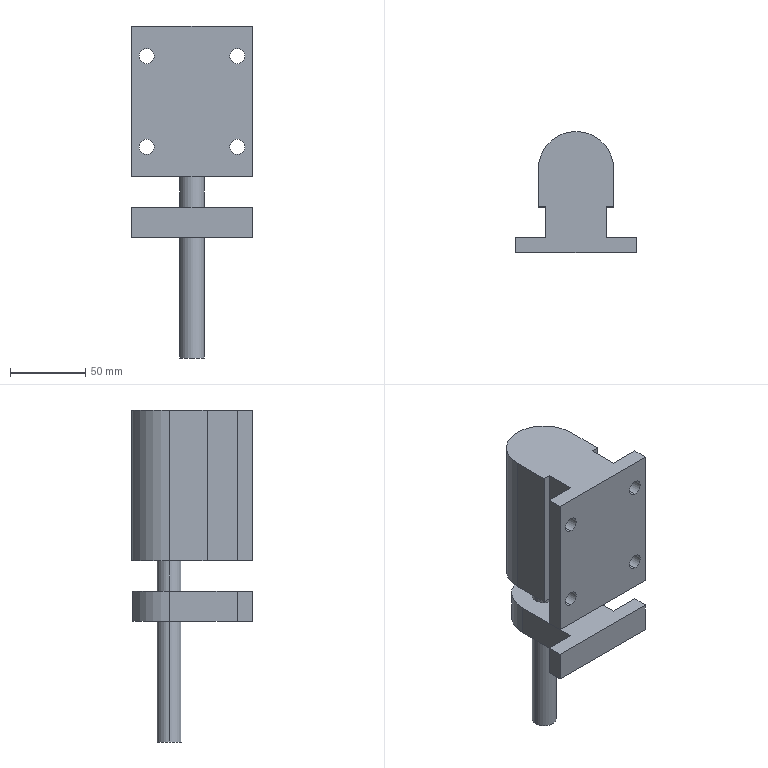Part | SolidWorks | features BaseBody 1 | 1 solid | 39 faces | box 80 x 80 x 220 mm | volume 466808 mm3 | plane 23 | cylinder 16 | commonest cylinder face diameters 10 x8 16 x4 50 x4
STEP:
#1=CARTESIAN_POINT('',(-246.782,7.138,175.));
#2=VERTEX_POINT('',#1);
#3=CARTESIAN_POINT('',(-246.782,7.138,165.));
#4=VERTEX_POINT('',#3);
#5=CARTESIAN_POINT('',(-246.782,7.138,170.));
#6=DIRECTION('',(0.,-1.,0.));
#7=DIRECTION('',(0.,0.,1.));
#8=AXIS2_PLACEMENT_3D('',#5,#6,#7);
#9=CIRCLE('',#8,5.);
#10=EDGE_CURVE('',#2,#4,#9,.T.);
#11=ORIENTED_EDGE('',*,*,#10,.T.);
#12=CARTESIAN_POINT('',(-246.782,17.138,165.));
#13=VERTEX_POINT('',#12);
#14=CARTESIAN_POINT('',(-246.782,-2.862,165.));
#15=DIRECTION('',(0.,1.,0.));
#16=VECTOR('',#15,1000.);
#17=LINE('',#14,#16);
#18=EDGE_CURVE('',#4,#13,#17,.T.);
#19=ORIENTED_EDGE('',*,*,#18,.T.);
#20=CARTESIAN_POINT('',(-246.782,17.138,175.));
#21=VERTEX_POINT('',#20);
#22=CARTESIAN_POINT('',(-246.782,17.138,170.));
#23=DIRECTION('',(0.,1.,0.));
#24=DIRECTION('',(0.,0.,1.));
#25=AXIS2_PLACEMENT_3D('',#22,#23,#24);
#26=CIRCLE('',#25,5.);
#27=EDGE_CURVE('',#13,#21,#26,.T.);
#28=ORIENTED_EDGE('',*,*,#27,.T.);
#29=CARTESIAN_POINT('',(-246.782,-2.862,175.));
#30=DIRECTION('',(0.,1.,0.));
#31=VECTOR('',#30,1000.);
#32=LINE('',#29,#31);
#33=EDGE_CURVE('',#2,#21,#32,.T.);
#34=ORIENTED_EDGE('',*,*,#33,.F.);
#35=EDGE_LOOP('',(#11,#19,#28,#34));
#36=FACE_OUTER_BOUND('',#35,.T.);
#37=CARTESIAN_POINT('',(-246.782,-2.862,170.));
#38=DIRECTION('',(0.,1.,0.));
#39=DIRECTION('',(0.,0.,1.));
#40=AXIS2_PLACEMENT_3D('',#37,#38,#39);
#41=CYLINDRICAL_SURFACE('',#40,5.);
#42=ADVANCED_FACE('',(#36),#41,.F.);
#43=CARTESIAN_POINT('',(-246.782,7.138,115.));
#44=VERTEX_POINT('',#43);
#45=CARTESIAN_POINT('',(-246.782,7.138,105.));
#46=VERTEX_POINT('',#45);
#47=CARTESIAN_POINT('',(-246.782,7.138,110.));
#48=DIRECTION('',(0.,-1.,0.));
#49=DIRECTION('',(0.,0.,1.));
#50=AXIS2_PLACEMENT_3D('',#47,#48,#49);
#51=CIRCLE('',#50,5.);
#52=EDGE_CURVE('',#44,#46,#51,.T.);
#53=ORIENTED_EDGE('',*,*,#52,.T.);
#54=CARTESIAN_POINT('',(-246.782,17.138,105.));
#55=VERTEX_POINT('',#54);
#56=CARTESIAN_POINT('',(-246.782,-2.862,105.));
#57=DIRECTION('',(0.,1.,0.));
#58=VECTOR('',#57,1000.);
#59=LINE('',#56,#58);
#60=EDGE_CURVE('',#46,#55,#59,.T.);
#61=ORIENTED_EDGE('',*,*,#60,.T.);
#62=CARTESIAN_POINT('',(-246.782,17.138,115.));
#63=VERTEX_POINT('',#62);
#64=CARTESIAN_POINT('',(-246.782,17.138,110.));
#65=DIRECTION('',(0.,1.,0.));
#66=DIRECTION('',(0.,0.,1.));
#67=AXIS2_PLACEMENT_3D('',#64,#65,#66);
#68=CIRCLE('',#67,5.);
#69=EDGE_CURVE('',#55,#63,#68,.T.);
#70=ORIENTED_EDGE('',*,*,#69,.T.);
#71=CARTESIAN_POINT('',(-246.782,-2.862,115.));
#72=DIRECTION('',(0.,1.,0.));
#73=VECTOR('',#72,1000.);
#74=LINE('',#71,#73);
#75=EDGE_CURVE('',#44,#63,#74,.T.);
#76=ORIENTED_EDGE('',*,*,#75,.F.);
#77=EDGE_LOOP('',(#53,#61,#70,#76));
#78=FACE_OUTER_BOUND('',#77,.T.);
#79=CARTESIAN_POINT('',(-246.782,-2.862,110.));
#80=DIRECTION('',(0.,1.,0.));
#81=DIRECTION('',(0.,0.,1.));
#82=AXIS2_PLACEMENT_3D('',#79,#80,#81);
#83=CYLINDRICAL_SURFACE('',#82,5.);
#84=ADVANCED_FACE('',(#78),#83,.F.);
#85=CARTESIAN_POINT('',(-306.782,7.138,115.));
#86=VERTEX_POINT('',#85);
#87=CARTESIAN_POINT('',(-306.782,7.138,105.));
#88=VERTEX_POINT('',#87);
#89=CARTESIAN_POINT('',(-306.782,7.138,110.));
#90=DIRECTION('',(0.,-1.,0.));
#91=DIRECTION('',(0.,0.,1.));
#92=AXIS2_PLACEMENT_3D('',#89,#90,#91);
#93=CIRCLE('',#92,5.);
#94=EDGE_CURVE('',#86,#88,#93,.T.);
#95=ORIENTED_EDGE('',*,*,#94,.T.);
#96=CARTESIAN_POINT('',(-306.782,17.138,105.));
#97=VERTEX_POINT('',#96);
#98=CARTESIAN_POINT('',(-306.782,-2.862,105.));
#99=DIRECTION('',(0.,1.,0.));
#100=VECTOR('',#99,1000.);
#101=LINE('',#98,#100);
#102=EDGE_CURVE('',#88,#97,#101,.T.);
#103=ORIENTED_EDGE('',*,*,#102,.T.);
#104=CARTESIAN_POINT('',(-306.782,17.138,115.));
#105=VERTEX_POINT('',#104);
#106=CARTESIAN_POINT('',(-306.782,17.138,110.));
#107=DIRECTION('',(0.,1.,0.));
#108=DIRECTION('',(0.,0.,-1.));
#109=AXIS2_PLACEMENT_3D('',#106,#107,#108);
#110=CIRCLE('',#109,5.);
#111=EDGE_CURVE('',#97,#105,#110,.T.);
#112=ORIENTED_EDGE('',*,*,#111,.T.);
#113=CARTESIAN_POINT('',(-306.782,-2.862,115.));
#114=DIRECTION('',(0.,1.,0.));
#115=VECTOR('',#114,1000.);
#116=LINE('',#113,#115);
#117=EDGE_CURVE('',#86,#105,#116,.T.);
#118=ORIENTED_EDGE('',*,*,#117,.F.);
#119=EDGE_LOOP('',(#95,#103,#112,#118));
#120=FACE_OUTER_BOUND('',#119,.T.);
#121=CARTESIAN_POINT('',(-306.782,-2.862,110.));
#122=DIRECTION('',(0.,1.,0.));
#123=DIRECTION('',(0.,0.,1.));
#124=AXIS2_PLACEMENT_3D('',#121,#122,#123);
#125=CYLINDRICAL_SURFACE('',#124,5.);
#126=ADVANCED_FACE('',(#120),#125,.F.);
#127=CARTESIAN_POINT('',(-306.782,7.138,175.));
#128=VERTEX_POINT('',#127);
#129=CARTESIAN_POINT('',(-306.782,7.138,165.));
#130=VERTEX_POINT('',#129);
#131=CARTESIAN_POINT('',(-306.782,7.138,170.));
#132=DIRECTION('',(0.,-1.,0.));
#133=DIRECTION('',(0.,0.,1.));
#134=AXIS2_PLACEMENT_3D('',#131,#132,#133);
#135=CIRCLE('',#134,5.);
#136=EDGE_CURVE('',#128,#130,#135,.T.);
#137=ORIENTED_EDGE('',*,*,#136,.T.);
#138=CARTESIAN_POINT('',(-306.782,17.138,165.));
#139=VERTEX_POINT('',#138);
#140=CARTESIAN_POINT('',(-306.782,-2.862,165.));
#141=DIRECTION('',(0.,1.,0.));
#142=VECTOR('',#141,1000.);
#143=LINE('',#140,#142);
#144=EDGE_CURVE('',#130,#139,#143,.T.);
#145=ORIENTED_EDGE('',*,*,#144,.T.);
#146=CARTESIAN_POINT('',(-306.782,17.138,175.));
#147=VERTEX_POINT('',#146);
#148=CARTESIAN_POINT('',(-306.782,17.138,170.));
#149=DIRECTION('',(0.,1.,0.));
#150=DIRECTION('',(0.,0.,-1.));
#151=AXIS2_PLACEMENT_3D('',#148,#149,#150);
#152=CIRCLE('',#151,5.);
#153=EDGE_CURVE('',#139,#147,#152,.T.);
#154=ORIENTED_EDGE('',*,*,#153,.T.);
#155=CARTESIAN_POINT('',(-306.782,-2.862,175.));
#156=DIRECTION('',(0.,1.,0.));
#157=VECTOR('',#156,1000.);
#158=LINE('',#155,#157);
#159=EDGE_CURVE('',#128,#147,#158,.T.);
#160=ORIENTED_EDGE('',*,*,#159,.F.);
#161=EDGE_LOOP('',(#137,#145,#154,#160));
#162=FACE_OUTER_BOUND('',#161,.T.);
#163=CARTESIAN_POINT('',(-306.782,-2.862,170.));
#164=DIRECTION('',(0.,1.,0.));
#165=DIRECTION('',(0.,0.,1.));
#166=AXIS2_PLACEMENT_3D('',#163,#164,#165);
#167=CYLINDRICAL_SURFACE('',#166,5.);
#168=ADVANCED_FACE('',(#162),#167,.F.);
#169=CARTESIAN_POINT('',(-284.782,62.138,90.));
#170=VERTEX_POINT('',#169);
#171=CARTESIAN_POINT('',(-268.782,62.138,90.));
#172=VERTEX_POINT('',#171);
#173=CARTESIAN_POINT('',(-276.782,62.138,90.));
#174=DIRECTION('',(0.,0.,-1.));
#175=DIRECTION('',(1.,0.,0.));
#176=AXIS2_PLACEMENT_3D('',#173,#174,#175);
#177=CIRCLE('',#176,8.);
#178=EDGE_CURVE('',#170,#172,#177,.T.);
#179=ORIENTED_EDGE('',*,*,#178,.T.);
#180=CARTESIAN_POINT('',(-268.782,62.138,70.));
#181=VERTEX_POINT('',#180);
#182=CARTESIAN_POINT('',(-268.782,62.138,112.627));
#183=DIRECTION('',(0.,0.,-1.));
#184=VECTOR('',#183,1000.);
#185=LINE('',#182,#184);
#186=EDGE_CURVE('',#172,#181,#185,.T.);
#187=ORIENTED_EDGE('',*,*,#186,.T.);
#188=CARTESIAN_POINT('',(-284.782,62.138,70.));
#189=VERTEX_POINT('',#188);
#190=CARTESIAN_POINT('',(-276.782,62.138,70.));
#191=DIRECTION('',(0.,0.,-1.));
#192=DIRECTION('',(-1.,0.,0.));
#193=AXIS2_PLACEMENT_3D('',#190,#191,#192);
#194=CIRCLE('',#193,8.);
#195=EDGE_CURVE('',#189,#181,#194,.T.);
#196=ORIENTED_EDGE('',*,*,#195,.F.);
#197=CARTESIAN_POINT('',(-284.782,62.138,112.627));
#198=DIRECTION('',(0.,0.,-1.));
#199=VECTOR('',#198,1000.);
#200=LINE('',#197,#199);
#201=EDGE_CURVE('',#170,#189,#200,.T.);
#202=ORIENTED_EDGE('',*,*,#201,.F.);
#203=EDGE_LOOP('',(#179,#187,#196,#202));
#204=FACE_OUTER_BOUND('',#203,.T.);
#205=CARTESIAN_POINT('',(-276.782,62.138,112.627));
#206=DIRECTION('',(0.,0.,-1.));
#207=DIRECTION('',(-1.,0.,0.));
#208=AXIS2_PLACEMENT_3D('',#205,#206,#207);
#209=CYLINDRICAL_SURFACE('',#208,8.);
#210=ADVANCED_FACE('',(#204),#209,.T.);
#211=CARTESIAN_POINT('',(-284.782,62.138,-30.));
#212=VERTEX_POINT('',#211);
#213=CARTESIAN_POINT('',(-268.782,62.138,-30.));
#214=VERTEX_POINT('',#213);
#215=CARTESIAN_POINT('',(-276.782,62.138,-30.));
#216=DIRECTION('',(0.,0.,-1.));
#217=DIRECTION('',(-1.,0.,0.));
#218=AXIS2_PLACEMENT_3D('',#215,#216,#217);
#219=CIRCLE('',#218,8.);
#220=EDGE_CURVE('',#212,#214,#219,.T.);
#221=ORIENTED_EDGE('',*,*,#220,.F.);
#222=CARTESIAN_POINT('',(-284.782,62.138,50.));
#223=VERTEX_POINT('',#222);
#224=CARTESIAN_POINT('',(-284.782,62.138,-30.));
#225=DIRECTION('',(0.,0.,1.));
#226=VECTOR('',#225,1000.);
#227=LINE('',#224,#226);
#228=EDGE_CURVE('',#212,#223,#227,.T.);
#229=ORIENTED_EDGE('',*,*,#228,.T.);
#230=CARTESIAN_POINT('',(-268.782,62.138,50.));
#231=VERTEX_POINT('',#230);
#232=CARTESIAN_POINT('',(-276.782,62.138,50.));
#233=DIRECTION('',(0.,0.,-1.));
#234=DIRECTION('',(1.,0.,0.));
#235=AXIS2_PLACEMENT_3D('',#232,#233,#234);
#236=CIRCLE('',#235,8.);
#237=EDGE_CURVE('',#223,#231,#236,.T.);
#238=ORIENTED_EDGE('',*,*,#237,.T.);
#239=CARTESIAN_POINT('',(-268.782,62.138,-30.));
#240=DIRECTION('',(0.,0.,1.));
#241=VECTOR('',#240,1000.);
#242=LINE('',#239,#241);
#243=EDGE_CURVE('',#214,#231,#242,.T.);
#244=ORIENTED_EDGE('',*,*,#243,.F.);
#245=EDGE_LOOP('',(#221,#229,#238,#244));
#246=FACE_OUTER_BOUND('',#245,.T.);
#247=CARTESIAN_POINT('',(-276.782,62.138,-30.));
#248=DIRECTION('',(0.,0.,1.));
#249=DIRECTION('',(1.,0.,0.));
#250=AXIS2_PLACEMENT_3D('',#247,#248,#249);
#251=CYLINDRICAL_SURFACE('',#250,8.);
#252=ADVANCED_FACE('',(#246),#251,.T.);
#253=CARTESIAN_POINT('',(-276.782,62.138,-30.));
#254=DIRECTION('',(0.,0.,-1.));
#255=DIRECTION('',(-1.,0.,0.));
#256=AXIS2_PLACEMENT_3D('',#253,#254,#255);
#257=CIRCLE('',#256,8.);
#258=EDGE_CURVE('',#214,#212,#257,.T.);
#259=ORIENTED_EDGE('',*,*,#258,.T.);
#260=ORIENTED_EDGE('',*,*,#220,.T.);
#261=EDGE_LOOP('',(#259,#260));
#262=FACE_OUTER_BOUND('',#261,.T.);
#263=CARTESIAN_POINT('',(-276.782,62.138,-30.));
#264=DIRECTION('',(0.,0.,-1.));
#265=DIRECTION('',(-1.,0.,0.));
#266=AXIS2_PLACEMENT_3D('',#263,#264,#265);
#267=PLANE('',#266);
#268=ADVANCED_FACE('',(#262),#267,.T.);
#269=ORIENTED_EDGE('',*,*,#228,.F.);
#270=ORIENTED_EDGE('',*,*,#258,.F.);
#271=ORIENTED_EDGE('',*,*,#243,.T.);
#272=CARTESIAN_POINT('',(-276.782,62.138,50.));
#273=DIRECTION('',(0.,0.,-1.));
#274=DIRECTION('',(1.,0.,0.));
#275=AXIS2_PLACEMENT_3D('',#272,#273,#274);
#276=CIRCLE('',#275,8.);
#277=EDGE_CURVE('',#231,#223,#276,.T.);
#278=ORIENTED_EDGE('',*,*,#277,.T.);
#279=EDGE_LOOP('',(#269,#270,#271,#278));
#280=FACE_OUTER_BOUND('',#279,.T.);
#281=CARTESIAN_POINT('',(-276.782,62.138,-30.));
#282=DIRECTION('',(0.,0.,1.));
#283=DIRECTION('',(1.,0.,0.));
#284=AXIS2_PLACEMENT_3D('',#281,#282,#283);
#285=CYLINDRICAL_SURFACE('',#284,8.);
#286=ADVANCED_FACE('',(#280),#285,.T.);
#287=CARTESIAN_POINT('',(-296.782,37.138,90.));
#288=VERTEX_POINT('',#287);
#289=CARTESIAN_POINT('',(-301.782,37.138,90.));
#290=VERTEX_POINT('',#289);
#291=CARTESIAN_POINT('',(-251.782,37.138,90.));
#292=DIRECTION('',(-1.,0.,0.));
#293=VECTOR('',#292,1000.);
#294=LINE('',#291,#293);
#295=EDGE_CURVE('',#288,#290,#294,.T.);
#296=ORIENTED_EDGE('',*,*,#295,.F.);
#297=CARTESIAN_POINT('',(-296.782,37.138,190.));
#298=VERTEX_POINT('',#297);
#299=CARTESIAN_POINT('',(-296.782,37.138,190.));
#300=DIRECTION('',(0.,0.,1.));
#301=VECTOR('',#300,1000.);
#302=LINE('',#299,#301);
#303=EDGE_CURVE('',#288,#298,#302,.T.);
#304=ORIENTED_EDGE('',*,*,#303,.T.);
#305=CARTESIAN_POINT('',(-301.782,37.138,190.));
#306=VERTEX_POINT('',#305);
#307=CARTESIAN_POINT('',(-301.782,37.138,190.));
#308=DIRECTION('',(1.,0.,0.));
#309=VECTOR('',#308,1000.);
#310=LINE('',#307,#309);
#311=EDGE_CURVE('',#306,#298,#310,.T.);
#312=ORIENTED_EDGE('',*,*,#311,.F.);
#313=CARTESIAN_POINT('',(-301.782,37.138,90.));
#314=DIRECTION('',(0.,0.,1.));
#315=VECTOR('',#314,1000.);
#316=LINE('',#313,#315);
#317=EDGE_CURVE('',#290,#306,#316,.T.);
#318=ORIENTED_EDGE('',*,*,#317,.F.);
#319=EDGE_LOOP('',(#296,#304,#312,#318));
#320=FACE_OUTER_BOUND('',#319,.T.);
#321=CARTESIAN_POINT('',(-616.782,37.138,0.));
#322=DIRECTION('',(0.,1.,0.));
#323=DIRECTION('',(0.,0.,1.));
#324=AXIS2_PLACEMENT_3D('',#321,#322,#323);
#325=PLANE('',#324);
#326=ADVANCED_FACE('',(#320),#325,.F.);
#327=CARTESIAN_POINT('',(-296.782,17.138,90.));
#328=VERTEX_POINT('',#327);
#329=CARTESIAN_POINT('',(-296.782,17.138,190.));
#330=VERTEX_POINT('',#329);
#331=CARTESIAN_POINT('',(-296.782,17.138,190.));
#332=DIRECTION('',(0.,0.,1.));
#333=VECTOR('',#332,1000.);
#334=LINE('',#331,#333);
#335=EDGE_CURVE('',#328,#330,#334,.T.);
#336=ORIENTED_EDGE('',*,*,#335,.T.);
#337=CARTESIAN_POINT('',(-296.782,37.138,190.));
#338=DIRECTION('',(0.,-1.,0.));
#339=VECTOR('',#338,1000.);
#340=LINE('',#337,#339);
#341=EDGE_CURVE('',#298,#330,#340,.T.);
#342=ORIENTED_EDGE('',*,*,#341,.F.);
#343=ORIENTED_EDGE('',*,*,#303,.F.);
#344=CARTESIAN_POINT('',(-296.782,37.138,90.));
#345=DIRECTION('',(0.,-1.,0.));
#346=VECTOR('',#345,1000.);
#347=LINE('',#344,#346);
#348=EDGE_CURVE('',#288,#328,#347,.T.);
#349=ORIENTED_EDGE('',*,*,#348,.T.);
#350=EDGE_LOOP('',(#336,#342,#343,#349));
#351=FACE_OUTER_BOUND('',#350,.T.);
#352=CARTESIAN_POINT('',(-296.782,37.138,190.));
#353=DIRECTION('',(1.,0.,0.));
#354=DIRECTION('',(0.,0.,-1.));
#355=AXIS2_PLACEMENT_3D('',#352,#353,#354);
#356=PLANE('',#355);
#357=ADVANCED_FACE('',(#351),#356,.F.);
#358=CARTESIAN_POINT('',(-256.782,17.138,190.));
#359=VERTEX_POINT('',#358);
#360=CARTESIAN_POINT('',(-256.782,17.138,90.));
#361=VERTEX_POINT('',#360);
#362=CARTESIAN_POINT('',(-256.782,17.138,90.));
#363=DIRECTION('',(0.,0.,-1.));
#364=VECTOR('',#363,1000.);
#365=LINE('',#362,#364);
#366=EDGE_CURVE('',#359,#361,#365,.T.);
#367=ORIENTED_EDGE('',*,*,#366,.T.);
#368=CARTESIAN_POINT('',(-256.782,37.138,90.));
#369=VERTEX_POINT('',#368);
#370=CARTESIAN_POINT('',(-256.782,37.138,90.));
#371=DIRECTION('',(0.,-1.,0.));
#372=VECTOR('',#371,1000.);
#373=LINE('',#370,#372);
#374=EDGE_CURVE('',#369,#361,#373,.T.);
#375=ORIENTED_EDGE('',*,*,#374,.F.);
#376=CARTESIAN_POINT('',(-256.782,37.138,190.));
#377=VERTEX_POINT('',#376);
#378=CARTESIAN_POINT('',(-256.782,37.138,90.));
#379=DIRECTION('',(0.,0.,-1.));
#380=VECTOR('',#379,1000.);
#381=LINE('',#378,#380);
#382=EDGE_CURVE('',#377,#369,#381,.T.);
#383=ORIENTED_EDGE('',*,*,#382,.F.);
#384=CARTESIAN_POINT('',(-256.782,37.138,190.));
#385=DIRECTION('',(0.,-1.,0.));
#386=VECTOR('',#385,1000.);
#387=LINE('',#384,#386);
#388=EDGE_CURVE('',#377,#359,#387,.T.);
#389=ORIENTED_EDGE('',*,*,#388,.T.);
#390=EDGE_LOOP('',(#367,#375,#383,#389));
#391=FACE_OUTER_BOUND('',#390,.T.);
#392=CARTESIAN_POINT('',(-256.782,37.138,90.));
#393=DIRECTION('',(-1.,0.,0.));
#394=DIRECTION('',(0.,0.,1.));
#395=AXIS2_PLACEMENT_3D('',#392,#393,#394);
#396=PLANE('',#395);
#397=ADVANCED_FACE('',(#391),#396,.F.);
#398=CARTESIAN_POINT('',(-251.782,37.138,190.));
#399=VERTEX_POINT('',#398);
#400=CARTESIAN_POINT('',(-301.782,37.138,190.));
#401=DIRECTION('',(1.,0.,0.));
#402=VECTOR('',#401,1000.);
#403=LINE('',#400,#402);
#404=EDGE_CURVE('',#377,#399,#403,.T.);
#405=ORIENTED_EDGE('',*,*,#404,.F.);
#406=ORIENTED_EDGE('',*,*,#382,.T.);
#407=CARTESIAN_POINT('',(-251.782,37.138,90.));
#408=VERTEX_POINT('',#407);
#409=CARTESIAN_POINT('',(-251.782,37.138,90.));
#410=DIRECTION('',(-1.,0.,0.));
#411=VECTOR('',#410,1000.);
#412=LINE('',#409,#411);
#413=EDGE_CURVE('',#408,#369,#412,.T.);
#414=ORIENTED_EDGE('',*,*,#413,.F.);
#415=CARTESIAN_POINT('',(-251.782,37.138,190.));
#416=DIRECTION('',(0.,0.,-1.));
#417=VECTOR('',#416,1000.);
#418=LINE('',#415,#417);
#419=EDGE_CURVE('',#399,#408,#418,.T.);
#420=ORIENTED_EDGE('',*,*,#419,.F.);
#421=EDGE_LOOP('',(#405,#406,#414,#420));
#422=FACE_OUTER_BOUND('',#421,.T.);
#423=CARTESIAN_POINT('',(-616.782,37.138,0.));
#424=DIRECTION('',(0.,1.,0.));
#425=DIRECTION('',(0.,0.,1.));
#426=AXIS2_PLACEMENT_3D('',#423,#424,#425);
#427=PLANE('',#426);
#428=ADVANCED_FACE('',(#422),#427,.F.);
#429=CARTESIAN_POINT('',(-251.782,62.138,90.));
#430=VERTEX_POINT('',#429);
#431=CARTESIAN_POINT('',(-251.782,87.138,90.));
#432=DIRECTION('',(0.,-1.,0.));
#433=VECTOR('',#432,1000.);
#434=LINE('',#431,#433);
#435=EDGE_CURVE('',#430,#408,#434,.T.);
#436=ORIENTED_EDGE('',*,*,#435,.F.);
#437=CARTESIAN_POINT('',(-251.782,62.138,190.));
#438=VERTEX_POINT('',#437);
#439=CARTESIAN_POINT('',(-251.782,62.138,190.));
#440=DIRECTION('',(0.,0.,1.));
#441=VECTOR('',#440,1000.);
#442=LINE('',#439,#441);
#443=EDGE_CURVE('',#430,#438,#442,.T.);
#444=ORIENTED_EDGE('',*,*,#443,.T.);
#445=CARTESIAN_POINT('',(-251.782,87.138,190.));
#446=DIRECTION('',(0.,-1.,0.));
#447=VECTOR('',#446,1000.);
#448=LINE('',#445,#447);
#449=EDGE_CURVE('',#438,#399,#448,.T.);
#450=ORIENTED_EDGE('',*,*,#449,.T.);
#451=ORIENTED_EDGE('',*,*,#419,.T.);
#452=EDGE_LOOP('',(#436,#444,#450,#451));
#453=FACE_OUTER_BOUND('',#452,.T.);
#454=CARTESIAN_POINT('',(-251.782,87.138,190.));
#455=DIRECTION('',(-1.,0.,0.));
#456=DIRECTION('',(0.,0.,1.));
#457=AXIS2_PLACEMENT_3D('',#454,#455,#456);
#458=PLANE('',#457);
#459=ADVANCED_FACE('',(#453),#458,.F.);
#460=ORIENTED_EDGE('',*,*,#443,.F.);
#461=CARTESIAN_POINT('',(-276.782,87.138,90.));
#462=VERTEX_POINT('',#461);
#463=CARTESIAN_POINT('',(-276.782,62.138,90.));
#464=DIRECTION('',(0.,0.,-1.));
#465=DIRECTION('',(1.,0.,0.));
#466=AXIS2_PLACEMENT_3D('',#463,#464,#465);
#467=CIRCLE('',#466,25.);
#468=EDGE_CURVE('',#462,#430,#467,.T.);
#469=ORIENTED_EDGE('',*,*,#468,.F.);
#470=CARTESIAN_POINT('',(-276.782,87.138,190.));
#471=VERTEX_POINT('',#470);
#472=CARTESIAN_POINT('',(-276.782,87.138,90.));
#473=DIRECTION('',(0.,0.,-1.));
#474=VECTOR('',#473,1000.);
#475=LINE('',#472,#474);
#476=EDGE_CURVE('',#471,#462,#475,.T.);
#477=ORIENTED_EDGE('',*,*,#476,.F.);
#478=CARTESIAN_POINT('',(-276.782,62.138,190.));
#479=DIRECTION('',(0.,0.,1.));
#480=DIRECTION('',(-1.,0.,0.));
#481=AXIS2_PLACEMENT_3D('',#478,#479,#480);
#482=CIRCLE('',#481,25.);
#483=EDGE_CURVE('',#438,#471,#482,.T.);
#484=ORIENTED_EDGE('',*,*,#483,.F.);
#485=EDGE_LOOP('',(#460,#469,#477,#484));
#486=FACE_OUTER_BOUND('',#485,.T.);
#487=CARTESIAN_POINT('',(-276.782,62.138,0.));
#488=DIRECTION('',(0.,0.,1.));
#489=DIRECTION('',(1.,0.,0.));
#490=AXIS2_PLACEMENT_3D('',#487,#488,#489);
#491=CYLINDRICAL_SURFACE('',#490,25.);
#492=ADVANCED_FACE('',(#486),#491,.T.);
#493=CARTESIAN_POINT('',(-301.782,62.138,90.));
#494=VERTEX_POINT('',#493);
#495=CARTESIAN_POINT('',(-276.782,62.138,90.));
#496=DIRECTION('',(0.,0.,-1.));
#497=DIRECTION('',(1.,0.,0.));
#498=AXIS2_PLACEMENT_3D('',#495,#496,#497);
#499=CIRCLE('',#498,25.);
#500=EDGE_CURVE('',#494,#462,#499,.T.);
#501=ORIENTED_EDGE('',*,*,#500,.F.);
#502=CARTESIAN_POINT('',(-301.782,62.138,190.));
#503=VERTEX_POINT('',#502);
#504=CARTESIAN_POINT('',(-301.782,62.138,90.));
#505=DIRECTION('',(0.,0.,-1.));
#506=VECTOR('',#505,1000.);
#507=LINE('',#504,#506);
#508=EDGE_CURVE('',#503,#494,#507,.T.);
#509=ORIENTED_EDGE('',*,*,#508,.F.);
#510=CARTESIAN_POINT('',(-276.782,62.138,190.));
#511=DIRECTION('',(0.,0.,1.));
#512=DIRECTION('',(-1.,0.,0.));
#513=AXIS2_PLACEMENT_3D('',#510,#511,#512);
#514=CIRCLE('',#513,25.);
#515=EDGE_CURVE('',#471,#503,#514,.T.);
#516=ORIENTED_EDGE('',*,*,#515,.F.);
#517=ORIENTED_EDGE('',*,*,#476,.T.);
#518=EDGE_LOOP('',(#501,#509,#516,#517));
#519=FACE_OUTER_BOUND('',#518,.T.);
#520=CARTESIAN_POINT('',(-276.782,62.138,0.));
#521=DIRECTION('',(0.,0.,-1.));
#522=DIRECTION('',(-1.,0.,0.));
#523=AXIS2_PLACEMENT_3D('',#520,#521,#522);
#524=CYLINDRICAL_SURFACE('',#523,25.);
#525=ADVANCED_FACE('',(#519),#524,.T.);
#526=CARTESIAN_POINT('',(-301.782,87.138,190.));
#527=DIRECTION('',(0.,-1.,0.));
#528=VECTOR('',#527,1000.);
#529=LINE('',#526,#528);
#530=EDGE_CURVE('',#503,#306,#529,.T.);
#531=ORIENTED_EDGE('',*,*,#530,.F.);
#532=ORIENTED_EDGE('',*,*,#508,.T.);
#533=CARTESIAN_POINT('',(-301.782,87.138,90.));
#534=DIRECTION('',(0.,-1.,0.));
#535=VECTOR('',#534,1000.);
#536=LINE('',#533,#535);
#537=EDGE_CURVE('',#494,#290,#536,.T.);
#538=ORIENTED_EDGE('',*,*,#537,.T.);
#539=ORIENTED_EDGE('',*,*,#317,.T.);
#540=EDGE_LOOP('',(#531,#532,#538,#539));
#541=FACE_OUTER_BOUND('',#540,.T.);
#542=CARTESIAN_POINT('',(-301.782,87.138,90.));
#543=DIRECTION('',(1.,0.,0.));
#544=DIRECTION('',(0.,0.,-1.));
#545=AXIS2_PLACEMENT_3D('',#542,#543,#544);
#546=PLANE('',#545);
#547=ADVANCED_FACE('',(#541),#546,.F.);
#548=CARTESIAN_POINT('',(-256.782,62.138,50.));
#549=VERTEX_POINT('',#548);
#550=CARTESIAN_POINT('',(-256.782,17.138,50.));
#551=VERTEX_POINT('',#550);
#552=CARTESIAN_POINT('',(-256.782,87.138,50.));
#553=DIRECTION('',(0.,-1.,0.));
#554=VECTOR('',#553,1000.);
#555=LINE('',#552,#554);
#556=EDGE_CURVE('',#549,#551,#555,.T.);
#557=ORIENTED_EDGE('',*,*,#556,.F.);
#558=CARTESIAN_POINT('',(-256.782,62.138,70.));
#559=VERTEX_POINT('',#558);
#560=CARTESIAN_POINT('',(-256.782,62.138,50.));
#561=DIRECTION('',(0.,0.,1.));
#562=VECTOR('',#561,1000.);
#563=LINE('',#560,#562);
#564=EDGE_CURVE('',#549,#559,#563,.T.);
#565=ORIENTED_EDGE('',*,*,#564,.T.);
#566=CARTESIAN_POINT('',(-256.782,17.138,70.));
#567=VERTEX_POINT('',#566);
#568=CARTESIAN_POINT('',(-256.782,87.138,70.));
#569=DIRECTION('',(0.,-1.,0.));
#570=VECTOR('',#569,1000.);
#571=LINE('',#568,#570);
#572=EDGE_CURVE('',#559,#567,#571,.T.);
#573=ORIENTED_EDGE('',*,*,#572,.T.);
#574=CARTESIAN_POINT('',(-256.782,17.138,50.));
#575=DIRECTION('',(0.,0.,-1.));
#576=VECTOR('',#575,1000.);
#577=LINE('',#574,#576);
#578=EDGE_CURVE('',#567,#551,#577,.T.);
#579=ORIENTED_EDGE('',*,*,#578,.T.);
#580=EDGE_LOOP('',(#557,#565,#573,#579));
#581=FACE_OUTER_BOUND('',#580,.T.);
#582=CARTESIAN_POINT('',(-256.782,87.138,50.));
#583=DIRECTION('',(-1.,0.,0.));
#584=DIRECTION('',(0.,0.,1.));
#585=AXIS2_PLACEMENT_3D('',#582,#583,#584);
#586=PLANE('',#585);
#587=ADVANCED_FACE('',(#581),#586,.F.);
#588=CARTESIAN_POINT('',(-296.782,17.138,50.));
#589=VERTEX_POINT('',#588);
#590=CARTESIAN_POINT('',(-296.782,17.138,70.));
#591=VERTEX_POINT('',#590);
#592=CARTESIAN_POINT('',(-296.782,17.138,70.));
#593=DIRECTION('',(0.,0.,1.));
#594=VECTOR('',#593,1000.);
#595=LINE('',#592,#594);
#596=EDGE_CURVE('',#589,#591,#595,.T.);
#597=ORIENTED_EDGE('',*,*,#596,.F.);
#598=CARTESIAN_POINT('',(-316.782,17.138,50.));
#599=VERTEX_POINT('',#598);
#600=CARTESIAN_POINT('',(-316.782,17.138,50.));
#601=DIRECTION('',(-1.,0.,0.));
#602=VECTOR('',#601,1000.);
#603=LINE('',#600,#602);
#604=EDGE_CURVE('',#589,#599,#603,.T.);
#605=ORIENTED_EDGE('',*,*,#604,.T.);
#606=CARTESIAN_POINT('',(-316.782,17.138,70.));
#607=VERTEX_POINT('',#606);
#608=CARTESIAN_POINT('',(-316.782,17.138,70.));
#609=DIRECTION('',(0.,0.,1.));
#610=VECTOR('',#609,1000.);
#611=LINE('',#608,#610);
#612=EDGE_CURVE('',#599,#607,#611,.T.);
#613=ORIENTED_EDGE('',*,*,#612,.T.);
#614=CARTESIAN_POINT('',(-316.782,17.138,70.));
#615=DIRECTION('',(1.,0.,0.));
#616=VECTOR('',#615,1000.);
#617=LINE('',#614,#616);
#618=EDGE_CURVE('',#607,#591,#617,.T.);
#619=ORIENTED_EDGE('',*,*,#618,.T.);
#620=EDGE_LOOP('',(#597,#605,#613,#619));
#621=FACE_OUTER_BOUND('',#620,.T.);
#622=CARTESIAN_POINT('',(-616.782,17.138,0.));
#623=DIRECTION('',(0.,-1.,0.));
#624=DIRECTION('',(0.,0.,-1.));
#625=AXIS2_PLACEMENT_3D('',#622,#623,#624);
#626=PLANE('',#625);
#627=ADVANCED_FACE('',(#621),#626,.F.);
#628=CARTESIAN_POINT('',(-296.782,62.138,70.));
#629=VERTEX_POINT('',#628);
#630=CARTESIAN_POINT('',(-296.782,87.138,70.));
#631=DIRECTION('',(0.,-1.,0.));
#632=VECTOR('',#631,1000.);
#633=LINE('',#630,#632);
#634=EDGE_CURVE('',#629,#591,#633,.T.);
#635=ORIENTED_EDGE('',*,*,#634,.F.);
#636=CARTESIAN_POINT('',(-296.782,62.138,50.));
#637=VERTEX_POINT('',#636);
#638=CARTESIAN_POINT('',(-296.782,62.138,70.));
#639=DIRECTION('',(0.,0.,-1.));
#640=VECTOR('',#639,1000.);
#641=LINE('',#638,#640);
#642=EDGE_CURVE('',#629,#637,#641,.T.);
#643=ORIENTED_EDGE('',*,*,#642,.T.);
#644=CARTESIAN_POINT('',(-296.782,87.138,50.));
#645=DIRECTION('',(0.,-1.,0.));
#646=VECTOR('',#645,1000.);
#647=LINE('',#644,#646);
#648=EDGE_CURVE('',#637,#589,#647,.T.);
#649=ORIENTED_EDGE('',*,*,#648,.T.);
#650=ORIENTED_EDGE('',*,*,#596,.T.);
#651=EDGE_LOOP('',(#635,#643,#649,#650));
#652=FACE_OUTER_BOUND('',#651,.T.);
#653=CARTESIAN_POINT('',(-296.782,87.138,70.));
#654=DIRECTION('',(1.,0.,0.));
#655=DIRECTION('',(0.,0.,-1.));
#656=AXIS2_PLACEMENT_3D('',#653,#654,#655);
#657=PLANE('',#656);
#658=ADVANCED_FACE('',(#652),#657,.F.);
#659=CARTESIAN_POINT('',(-276.782,86.633,50.));
#660=VERTEX_POINT('',#659);
#661=CARTESIAN_POINT('',(-271.782,62.138,50.));
#662=DIRECTION('',(0.,0.,-1.));
#663=DIRECTION('',(1.,0.,0.));
#664=AXIS2_PLACEMENT_3D('',#661,#662,#663);
#665=CIRCLE('',#664,25.);
#666=EDGE_CURVE('',#637,#660,#665,.T.);
#667=ORIENTED_EDGE('',*,*,#666,.F.);
#668=ORIENTED_EDGE('',*,*,#642,.F.);
#669=CARTESIAN_POINT('',(-276.782,86.633,70.));
#670=VERTEX_POINT('',#669);
#671=CARTESIAN_POINT('',(-271.782,62.138,70.));
#672=DIRECTION('',(0.,0.,1.));
#673=DIRECTION('',(-1.,0.,0.));
#674=AXIS2_PLACEMENT_3D('',#671,#672,#673);
#675=CIRCLE('',#674,25.);
#676=EDGE_CURVE('',#670,#629,#675,.T.);
#677=ORIENTED_EDGE('',*,*,#676,.F.);
#678=CARTESIAN_POINT('',(-276.782,86.633,60.));
#679=DIRECTION('',(0.,0.,-1.));
#680=VECTOR('',#679,1000.);
#681=LINE('',#678,#680);
#682=EDGE_CURVE('',#670,#660,#681,.T.);
#683=ORIENTED_EDGE('',*,*,#682,.T.);
#684=EDGE_LOOP('',(#667,#668,#677,#683));
#685=FACE_OUTER_BOUND('',#684,.T.);
#686=CARTESIAN_POINT('',(-271.782,62.138,0.));
#687=DIRECTION('',(0.,0.,1.));
#688=DIRECTION('',(1.,0.,0.));
#689=AXIS2_PLACEMENT_3D('',#686,#687,#688);
#690=CYLINDRICAL_SURFACE('',#689,25.);
#691=ADVANCED_FACE('',(#685),#690,.T.);
#692=ORIENTED_EDGE('',*,*,#564,.F.);
#693=CARTESIAN_POINT('',(-281.782,62.138,50.));
#694=DIRECTION('',(0.,0.,-1.));
#695=DIRECTION('',(1.,0.,0.));
#696=AXIS2_PLACEMENT_3D('',#693,#694,#695);
#697=CIRCLE('',#696,25.);
#698=EDGE_CURVE('',#660,#549,#697,.T.);
#699=ORIENTED_EDGE('',*,*,#698,.F.);
#700=ORIENTED_EDGE('',*,*,#682,.F.);
#701=CARTESIAN_POINT('',(-281.782,62.138,70.));
#702=DIRECTION('',(0.,0.,1.));
#703=DIRECTION('',(-1.,0.,0.));
#704=AXIS2_PLACEMENT_3D('',#701,#702,#703);
#705=CIRCLE('',#704,25.);
#706=EDGE_CURVE('',#559,#670,#705,.T.);
#707=ORIENTED_EDGE('',*,*,#706,.F.);
#708=EDGE_LOOP('',(#692,#699,#700,#707));
#709=FACE_OUTER_BOUND('',#708,.T.);
#710=CARTESIAN_POINT('',(-281.782,62.138,0.));
#711=DIRECTION('',(0.,0.,-1.));
#712=DIRECTION('',(-1.,0.,0.));
#713=AXIS2_PLACEMENT_3D('',#710,#711,#712);
#714=CYLINDRICAL_SURFACE('',#713,25.);
#715=ADVANCED_FACE('',(#709),#714,.T.);
#716=ORIENTED_EDGE('',*,*,#178,.F.);
#717=CARTESIAN_POINT('',(-276.782,62.138,90.));
#718=DIRECTION('',(0.,0.,-1.));
#719=DIRECTION('',(1.,0.,0.));
#720=AXIS2_PLACEMENT_3D('',#717,#718,#719);
#721=CIRCLE('',#720,8.);
#722=EDGE_CURVE('',#172,#170,#721,.T.);
#723=ORIENTED_EDGE('',*,*,#722,.F.);
#724=EDGE_LOOP('',(#716,#723));
#725=FACE_BOUND('',#724,.T.);
#726=ORIENTED_EDGE('',*,*,#537,.F.);
#727=ORIENTED_EDGE('',*,*,#500,.T.);
#728=ORIENTED_EDGE('',*,*,#468,.T.);
#729=ORIENTED_EDGE('',*,*,#435,.T.);
#730=ORIENTED_EDGE('',*,*,#413,.T.);
#731=ORIENTED_EDGE('',*,*,#374,.T.);
#732=CARTESIAN_POINT('',(-236.782,17.138,90.));
#733=VERTEX_POINT('',#732);
#734=CARTESIAN_POINT('',(-316.782,17.138,90.));
#735=DIRECTION('',(-1.,0.,0.));
#736=VECTOR('',#735,1000.);
#737=LINE('',#734,#736);
#738=EDGE_CURVE('',#733,#361,#737,.T.);
#739=ORIENTED_EDGE('',*,*,#738,.F.);
#740=CARTESIAN_POINT('',(-236.782,7.138,90.));
#741=VERTEX_POINT('',#740);
#742=CARTESIAN_POINT('',(-236.782,17.138,90.));
#743=DIRECTION('',(0.,-1.,0.));
#744=VECTOR('',#743,1000.);
#745=LINE('',#742,#744);
#746=EDGE_CURVE('',#733,#741,#745,.T.);
#747=ORIENTED_EDGE('',*,*,#746,.T.);
#748=CARTESIAN_POINT('',(-316.782,7.138,90.));
#749=VERTEX_POINT('',#748);
#750=CARTESIAN_POINT('',(-316.782,7.138,90.));
#751=DIRECTION('',(-1.,0.,0.));
#752=VECTOR('',#751,1000.);
#753=LINE('',#750,#752);
#754=EDGE_CURVE('',#741,#749,#753,.T.);
#755=ORIENTED_EDGE('',*,*,#754,.T.);
#756=CARTESIAN_POINT('',(-316.782,17.138,90.));
#757=VERTEX_POINT('',#756);
#758=CARTESIAN_POINT('',(-316.782,17.138,90.));
#759=DIRECTION('',(0.,-1.,0.));
#760=VECTOR('',#759,1000.);
#761=LINE('',#758,#760);
#762=EDGE_CURVE('',#757,#749,#761,.T.);
#763=ORIENTED_EDGE('',*,*,#762,.F.);
#764=CARTESIAN_POINT('',(-316.782,17.138,90.));
#765=DIRECTION('',(-1.,0.,0.));
#766=VECTOR('',#765,1000.);
#767=LINE('',#764,#766);
#768=EDGE_CURVE('',#328,#757,#767,.T.);
#769=ORIENTED_EDGE('',*,*,#768,.F.);
#770=ORIENTED_EDGE('',*,*,#348,.F.);
#771=ORIENTED_EDGE('',*,*,#295,.T.);
#772=EDGE_LOOP('',(#726,#727,#728,#729,#730,#731,#739,#747,#755,#763,#769,#770,#771));
#773=FACE_OUTER_BOUND('',#772,.T.);
#774=CARTESIAN_POINT('',(-316.782,17.138,90.));
#775=DIRECTION('',(0.,0.,1.));
#776=DIRECTION('',(1.,0.,0.));
#777=AXIS2_PLACEMENT_3D('',#774,#775,#776);
#778=PLANE('',#777);
#779=ADVANCED_FACE('',(#725,#773),#778,.F.);
#780=CARTESIAN_POINT('',(-236.782,7.138,190.));
#781=VERTEX_POINT('',#780);
#782=CARTESIAN_POINT('',(-236.782,7.138,90.));
#783=DIRECTION('',(0.,0.,-1.));
#784=VECTOR('',#783,1000.);
#785=LINE('',#782,#784);
#786=EDGE_CURVE('',#781,#741,#785,.T.);
#787=ORIENTED_EDGE('',*,*,#786,.T.);
#788=ORIENTED_EDGE('',*,*,#746,.F.);
#789=CARTESIAN_POINT('',(-236.782,17.138,190.));
#790=VERTEX_POINT('',#789);
#791=CARTESIAN_POINT('',(-236.782,17.138,90.));
#792=DIRECTION('',(0.,0.,-1.));
#793=VECTOR('',#792,1000.);
#794=LINE('',#791,#793);
#795=EDGE_CURVE('',#790,#733,#794,.T.);
#796=ORIENTED_EDGE('',*,*,#795,.F.);
#797=CARTESIAN_POINT('',(-236.782,17.138,190.));
#798=DIRECTION('',(0.,-1.,0.));
#799=VECTOR('',#798,1000.);
#800=LINE('',#797,#799);
#801=EDGE_CURVE('',#790,#781,#800,.T.);
#802=ORIENTED_EDGE('',*,*,#801,.T.);
#803=EDGE_LOOP('',(#787,#788,#796,#802));
#804=FACE_OUTER_BOUND('',#803,.T.);
#805=CARTESIAN_POINT('',(-236.782,17.138,90.));
#806=DIRECTION('',(-1.,0.,0.));
#807=DIRECTION('',(0.,0.,1.));
#808=AXIS2_PLACEMENT_3D('',#805,#806,#807);
#809=PLANE('',#808);
#810=ADVANCED_FACE('',(#804),#809,.F.);
#811=ORIENTED_EDGE('',*,*,#483,.T.);
#812=ORIENTED_EDGE('',*,*,#515,.T.);
#813=ORIENTED_EDGE('',*,*,#530,.T.);
#814=ORIENTED_EDGE('',*,*,#311,.T.);
#815=ORIENTED_EDGE('',*,*,#341,.T.);
#816=CARTESIAN_POINT('',(-316.782,17.138,190.));
#817=VERTEX_POINT('',#816);
#818=CARTESIAN_POINT('',(-236.782,17.138,190.));
#819=DIRECTION('',(1.,0.,0.));
#820=VECTOR('',#819,1000.);
#821=LINE('',#818,#820);
#822=EDGE_CURVE('',#817,#330,#821,.T.);
#823=ORIENTED_EDGE('',*,*,#822,.F.);
#824=CARTESIAN_POINT('',(-316.782,7.138,190.));
#825=VERTEX_POINT('',#824);
#826=CARTESIAN_POINT('',(-316.782,17.138,190.));
#827=DIRECTION('',(0.,-1.,0.));
#828=VECTOR('',#827,1000.);
#829=LINE('',#826,#828);
#830=EDGE_CURVE('',#817,#825,#829,.T.);
#831=ORIENTED_EDGE('',*,*,#830,.T.);
#832=CARTESIAN_POINT('',(-236.782,7.138,190.));
#833=DIRECTION('',(1.,0.,0.));
#834=VECTOR('',#833,1000.);
#835=LINE('',#832,#834);
#836=EDGE_CURVE('',#825,#781,#835,.T.);
#837=ORIENTED_EDGE('',*,*,#836,.T.);
#838=ORIENTED_EDGE('',*,*,#801,.F.);
#839=CARTESIAN_POINT('',(-236.782,17.138,190.));
#840=DIRECTION('',(1.,0.,0.));
#841=VECTOR('',#840,1000.);
#842=LINE('',#839,#841);
#843=EDGE_CURVE('',#359,#790,#842,.T.);
#844=ORIENTED_EDGE('',*,*,#843,.F.);
#845=ORIENTED_EDGE('',*,*,#388,.F.);
#846=ORIENTED_EDGE('',*,*,#404,.T.);
#847=ORIENTED_EDGE('',*,*,#449,.F.);
#848=EDGE_LOOP('',(#811,#812,#813,#814,#815,#823,#831,#837,#838,#844,#845,#846,#847));
#849=FACE_OUTER_BOUND('',#848,.T.);
#850=CARTESIAN_POINT('',(-236.782,17.138,190.));
#851=DIRECTION('',(0.,0.,-1.));
#852=DIRECTION('',(-1.,0.,0.));
#853=AXIS2_PLACEMENT_3D('',#850,#851,#852);
#854=PLANE('',#853);
#855=ADVANCED_FACE('',(#849),#854,.F.);
#856=CARTESIAN_POINT('',(-316.782,7.138,190.));
#857=DIRECTION('',(0.,0.,1.));
#858=VECTOR('',#857,1000.);
#859=LINE('',#856,#858);
#860=EDGE_CURVE('',#749,#825,#859,.T.);
#861=ORIENTED_EDGE('',*,*,#860,.T.);
#862=ORIENTED_EDGE('',*,*,#830,.F.);
#863=CARTESIAN_POINT('',(-316.782,17.138,190.));
#864=DIRECTION('',(0.,0.,1.));
#865=VECTOR('',#864,1000.);
#866=LINE('',#863,#865);
#867=EDGE_CURVE('',#757,#817,#866,.T.);
#868=ORIENTED_EDGE('',*,*,#867,.F.);
#869=ORIENTED_EDGE('',*,*,#762,.T.);
#870=EDGE_LOOP('',(#861,#862,#868,#869));
#871=FACE_OUTER_BOUND('',#870,.T.);
#872=CARTESIAN_POINT('',(-316.782,17.138,190.));
#873=DIRECTION('',(1.,0.,0.));
#874=DIRECTION('',(0.,0.,-1.));
#875=AXIS2_PLACEMENT_3D('',#872,#873,#874);
#876=PLANE('',#875);
#877=ADVANCED_FACE('',(#871),#876,.F.);
#878=ORIENTED_EDGE('',*,*,#186,.F.);
#879=ORIENTED_EDGE('',*,*,#722,.T.);
#880=ORIENTED_EDGE('',*,*,#201,.T.);
#881=CARTESIAN_POINT('',(-276.782,62.138,70.));
#882=DIRECTION('',(0.,0.,-1.));
#883=DIRECTION('',(-1.,0.,0.));
#884=AXIS2_PLACEMENT_3D('',#881,#882,#883);
#885=CIRCLE('',#884,8.);
#886=EDGE_CURVE('',#181,#189,#885,.T.);
#887=ORIENTED_EDGE('',*,*,#886,.F.);
#888=EDGE_LOOP('',(#878,#879,#880,#887));
#889=FACE_OUTER_BOUND('',#888,.T.);
#890=CARTESIAN_POINT('',(-276.782,62.138,112.627));
#891=DIRECTION('',(0.,0.,-1.));
#892=DIRECTION('',(-1.,0.,0.));
#893=AXIS2_PLACEMENT_3D('',#890,#891,#892);
#894=CYLINDRICAL_SURFACE('',#893,8.);
#895=ADVANCED_FACE('',(#889),#894,.T.);
#896=ORIENTED_EDGE('',*,*,#578,.F.);
#897=CARTESIAN_POINT('',(-236.782,17.138,70.));
#898=VERTEX_POINT('',#897);
#899=CARTESIAN_POINT('',(-316.782,17.138,70.));
#900=DIRECTION('',(1.,0.,0.));
#901=VECTOR('',#900,1000.);
#902=LINE('',#899,#901);
#903=EDGE_CURVE('',#567,#898,#902,.T.);
#904=ORIENTED_EDGE('',*,*,#903,.T.);
#905=CARTESIAN_POINT('',(-236.782,17.138,50.));
#906=VERTEX_POINT('',#905);
#907=CARTESIAN_POINT('',(-236.782,17.138,50.));
#908=DIRECTION('',(0.,0.,-1.));
#909=VECTOR('',#908,1000.);
#910=LINE('',#907,#909);
#911=EDGE_CURVE('',#898,#906,#910,.T.);
#912=ORIENTED_EDGE('',*,*,#911,.T.);
#913=CARTESIAN_POINT('',(-316.782,17.138,50.));
#914=DIRECTION('',(-1.,0.,0.));
#915=VECTOR('',#914,1000.);
#916=LINE('',#913,#915);
#917=EDGE_CURVE('',#906,#551,#916,.T.);
#918=ORIENTED_EDGE('',*,*,#917,.T.);
#919=EDGE_LOOP('',(#896,#904,#912,#918));
#920=FACE_OUTER_BOUND('',#919,.T.);
#921=CARTESIAN_POINT('',(-616.782,17.138,0.));
#922=DIRECTION('',(0.,-1.,0.));
#923=DIRECTION('',(0.,0.,-1.));
#924=AXIS2_PLACEMENT_3D('',#921,#922,#923);
#925=PLANE('',#924);
#926=ADVANCED_FACE('',(#920),#925,.F.);
#927=CARTESIAN_POINT('',(-236.782,7.138,70.));
#928=VERTEX_POINT('',#927);
#929=CARTESIAN_POINT('',(-236.782,7.138,50.));
#930=VERTEX_POINT('',#929);
#931=CARTESIAN_POINT('',(-236.782,7.138,50.));
#932=DIRECTION('',(0.,0.,-1.));
#933=VECTOR('',#932,1000.);
#934=LINE('',#931,#933);
#935=EDGE_CURVE('',#928,#930,#934,.T.);
#936=ORIENTED_EDGE('',*,*,#935,.T.);
#937=CARTESIAN_POINT('',(-236.782,17.138,50.));
#938=DIRECTION('',(0.,-1.,0.));
#939=VECTOR('',#938,1000.);
#940=LINE('',#937,#939);
#941=EDGE_CURVE('',#906,#930,#940,.T.);
#942=ORIENTED_EDGE('',*,*,#941,.F.);
#943=ORIENTED_EDGE('',*,*,#911,.F.);
#944=CARTESIAN_POINT('',(-236.782,17.138,70.));
#945=DIRECTION('',(0.,-1.,0.));
#946=VECTOR('',#945,1000.);
#947=LINE('',#944,#946);
#948=EDGE_CURVE('',#898,#928,#947,.T.);
#949=ORIENTED_EDGE('',*,*,#948,.T.);
#950=EDGE_LOOP('',(#936,#942,#943,#949));
#951=FACE_OUTER_BOUND('',#950,.T.);
#952=CARTESIAN_POINT('',(-236.782,17.138,50.));
#953=DIRECTION('',(-1.,0.,0.));
#954=DIRECTION('',(0.,0.,1.));
#955=AXIS2_PLACEMENT_3D('',#952,#953,#954);
#956=PLANE('',#955);
#957=ADVANCED_FACE('',(#951),#956,.F.);
#958=ORIENTED_EDGE('',*,*,#195,.T.);
#959=ORIENTED_EDGE('',*,*,#886,.T.);
#960=EDGE_LOOP('',(#958,#959));
#961=FACE_BOUND('',#960,.T.);
#962=ORIENTED_EDGE('',*,*,#706,.T.);
#963=ORIENTED_EDGE('',*,*,#676,.T.);
#964=ORIENTED_EDGE('',*,*,#634,.T.);
#965=ORIENTED_EDGE('',*,*,#618,.F.);
#966=CARTESIAN_POINT('',(-316.782,7.138,70.));
#967=VERTEX_POINT('',#966);
#968=CARTESIAN_POINT('',(-316.782,17.138,70.));
#969=DIRECTION('',(0.,-1.,0.));
#970=VECTOR('',#969,1000.);
#971=LINE('',#968,#970);
#972=EDGE_CURVE('',#607,#967,#971,.T.);
#973=ORIENTED_EDGE('',*,*,#972,.T.);
#974=CARTESIAN_POINT('',(-316.782,7.138,70.));
#975=DIRECTION('',(1.,0.,0.));
#976=VECTOR('',#975,1000.);
#977=LINE('',#974,#976);
#978=EDGE_CURVE('',#967,#928,#977,.T.);
#979=ORIENTED_EDGE('',*,*,#978,.T.);
#980=ORIENTED_EDGE('',*,*,#948,.F.);
#981=ORIENTED_EDGE('',*,*,#903,.F.);
#982=ORIENTED_EDGE('',*,*,#572,.F.);
#983=EDGE_LOOP('',(#962,#963,#964,#965,#973,#979,#980,#981,#982));
#984=FACE_OUTER_BOUND('',#983,.T.);
#985=CARTESIAN_POINT('',(-316.782,17.138,70.));
#986=DIRECTION('',(0.,0.,-1.));
#987=DIRECTION('',(-1.,0.,0.));
#988=AXIS2_PLACEMENT_3D('',#985,#986,#987);
#989=PLANE('',#988);
#990=ADVANCED_FACE('',(#961,#984),#989,.F.);
#991=CARTESIAN_POINT('',(-316.782,7.138,50.));
#992=VERTEX_POINT('',#991);
#993=CARTESIAN_POINT('',(-316.782,7.138,70.));
#994=DIRECTION('',(0.,0.,1.));
#995=VECTOR('',#994,1000.);
#996=LINE('',#993,#995);
#997=EDGE_CURVE('',#992,#967,#996,.T.);
#998=ORIENTED_EDGE('',*,*,#997,.T.);
#999=ORIENTED_EDGE('',*,*,#972,.F.);
#1000=ORIENTED_EDGE('',*,*,#612,.F.);
#1001=CARTESIAN_POINT('',(-316.782,17.138,50.));
#1002=DIRECTION('',(0.,-1.,0.));
#1003=VECTOR('',#1002,1000.);
#1004=LINE('',#1001,#1003);
#1005=EDGE_CURVE('',#599,#992,#1004,.T.);
#1006=ORIENTED_EDGE('',*,*,#1005,.T.);
#1007=EDGE_LOOP('',(#998,#999,#1000,#1006));
#1008=FACE_OUTER_BOUND('',#1007,.T.);
#1009=CARTESIAN_POINT('',(-316.782,17.138,70.));
#1010=DIRECTION('',(1.,0.,0.));
#1011=DIRECTION('',(0.,0.,-1.));
#1012=AXIS2_PLACEMENT_3D('',#1009,#1010,#1011);
#1013=PLANE('',#1012);
#1014=ADVANCED_FACE('',(#1008),#1013,.F.);
#1015=ORIENTED_EDGE('',*,*,#648,.F.);
#1016=ORIENTED_EDGE('',*,*,#666,.T.);
#1017=ORIENTED_EDGE('',*,*,#698,.T.);
#1018=ORIENTED_EDGE('',*,*,#556,.T.);
#1019=ORIENTED_EDGE('',*,*,#917,.F.);
#1020=ORIENTED_EDGE('',*,*,#941,.T.);
#1021=CARTESIAN_POINT('',(-316.782,7.138,50.));
#1022=DIRECTION('',(-1.,0.,0.));
#1023=VECTOR('',#1022,1000.);
#1024=LINE('',#1021,#1023);
#1025=EDGE_CURVE('',#930,#992,#1024,.T.);
#1026=ORIENTED_EDGE('',*,*,#1025,.T.);
#1027=ORIENTED_EDGE('',*,*,#1005,.F.);
#1028=ORIENTED_EDGE('',*,*,#604,.F.);
#1029=EDGE_LOOP('',(#1015,#1016,#1017,#1018,#1019,#1020,#1026,#1027,#1028));
#1030=FACE_OUTER_BOUND('',#1029,.T.);
#1031=ORIENTED_EDGE('',*,*,#277,.F.);
#1032=ORIENTED_EDGE('',*,*,#237,.F.);
#1033=EDGE_LOOP('',(#1031,#1032));
#1034=FACE_BOUND('',#1033,.T.);
#1035=CARTESIAN_POINT('',(-316.782,17.138,50.));
#1036=DIRECTION('',(0.,0.,1.));
#1037=DIRECTION('',(1.,0.,0.));
#1038=AXIS2_PLACEMENT_3D('',#1035,#1036,#1037);
#1039=PLANE('',#1038);
#1040=ADVANCED_FACE('',(#1030,#1034),#1039,.F.);
#1041=ORIENTED_EDGE('',*,*,#144,.F.);
#1042=CARTESIAN_POINT('',(-306.782,7.138,170.));
#1043=DIRECTION('',(0.,-1.,0.));
#1044=DIRECTION('',(0.,0.,1.));
#1045=AXIS2_PLACEMENT_3D('',#1042,#1043,#1044);
#1046=CIRCLE('',#1045,5.);
#1047=EDGE_CURVE('',#130,#128,#1046,.T.);
#1048=ORIENTED_EDGE('',*,*,#1047,.T.);
#1049=ORIENTED_EDGE('',*,*,#159,.T.);
#1050=CARTESIAN_POINT('',(-306.782,17.138,170.));
#1051=DIRECTION('',(0.,1.,0.));
#1052=DIRECTION('',(0.,0.,-1.));
#1053=AXIS2_PLACEMENT_3D('',#1050,#1051,#1052);
#1054=CIRCLE('',#1053,5.);
#1055=EDGE_CURVE('',#147,#139,#1054,.T.);
#1056=ORIENTED_EDGE('',*,*,#1055,.T.);
#1057=EDGE_LOOP('',(#1041,#1048,#1049,#1056));
#1058=FACE_OUTER_BOUND('',#1057,.T.);
#1059=CARTESIAN_POINT('',(-306.782,-2.862,170.));
#1060=DIRECTION('',(0.,1.,0.));
#1061=DIRECTION('',(0.,0.,1.));
#1062=AXIS2_PLACEMENT_3D('',#1059,#1060,#1061);
#1063=CYLINDRICAL_SURFACE('',#1062,5.);
#1064=ADVANCED_FACE('',(#1058),#1063,.F.);
#1065=CARTESIAN_POINT('',(-306.782,17.138,110.));
#1066=DIRECTION('',(0.,1.,0.));
#1067=DIRECTION('',(0.,0.,-1.));
#1068=AXIS2_PLACEMENT_3D('',#1065,#1066,#1067);
#1069=CIRCLE('',#1068,5.);
#1070=EDGE_CURVE('',#105,#97,#1069,.T.);
#1071=ORIENTED_EDGE('',*,*,#1070,.F.);
#1072=ORIENTED_EDGE('',*,*,#111,.F.);
#1073=EDGE_LOOP('',(#1071,#1072));
#1074=FACE_BOUND('',#1073,.T.);
#1075=ORIENTED_EDGE('',*,*,#1055,.F.);
#1076=ORIENTED_EDGE('',*,*,#153,.F.);
#1077=EDGE_LOOP('',(#1075,#1076));
#1078=FACE_BOUND('',#1077,.T.);
#1079=ORIENTED_EDGE('',*,*,#335,.F.);
#1080=ORIENTED_EDGE('',*,*,#768,.T.);
#1081=ORIENTED_EDGE('',*,*,#867,.T.);
#1082=ORIENTED_EDGE('',*,*,#822,.T.);
#1083=EDGE_LOOP('',(#1079,#1080,#1081,#1082));
#1084=FACE_OUTER_BOUND('',#1083,.T.);
#1085=CARTESIAN_POINT('',(-616.782,17.138,0.));
#1086=DIRECTION('',(0.,-1.,0.));
#1087=DIRECTION('',(0.,0.,-1.));
#1088=AXIS2_PLACEMENT_3D('',#1085,#1086,#1087);
#1089=PLANE('',#1088);
#1090=ADVANCED_FACE('',(#1074,#1078,#1084),#1089,.F.);
#1091=ORIENTED_EDGE('',*,*,#102,.F.);
#1092=CARTESIAN_POINT('',(-306.782,7.138,110.));
#1093=DIRECTION('',(0.,-1.,0.));
#1094=DIRECTION('',(0.,0.,1.));
#1095=AXIS2_PLACEMENT_3D('',#1092,#1093,#1094);
#1096=CIRCLE('',#1095,5.);
#1097=EDGE_CURVE('',#88,#86,#1096,.T.);
#1098=ORIENTED_EDGE('',*,*,#1097,.T.);
#1099=ORIENTED_EDGE('',*,*,#117,.T.);
#1100=ORIENTED_EDGE('',*,*,#1070,.T.);
#1101=EDGE_LOOP('',(#1091,#1098,#1099,#1100));
#1102=FACE_OUTER_BOUND('',#1101,.T.);
#1103=CARTESIAN_POINT('',(-306.782,-2.862,110.));
#1104=DIRECTION('',(0.,1.,0.));
#1105=DIRECTION('',(0.,0.,1.));
#1106=AXIS2_PLACEMENT_3D('',#1103,#1104,#1105);
#1107=CYLINDRICAL_SURFACE('',#1106,5.);
#1108=ADVANCED_FACE('',(#1102),#1107,.F.);
#1109=ORIENTED_EDGE('',*,*,#60,.F.);
#1110=CARTESIAN_POINT('',(-246.782,7.138,110.));
#1111=DIRECTION('',(0.,-1.,0.));
#1112=DIRECTION('',(0.,0.,1.));
#1113=AXIS2_PLACEMENT_3D('',#1110,#1111,#1112);
#1114=CIRCLE('',#1113,5.);
#1115=EDGE_CURVE('',#46,#44,#1114,.T.);
#1116=ORIENTED_EDGE('',*,*,#1115,.T.);
#1117=ORIENTED_EDGE('',*,*,#75,.T.);
#1118=CARTESIAN_POINT('',(-246.782,17.138,110.));
#1119=DIRECTION('',(0.,1.,0.));
#1120=DIRECTION('',(0.,0.,1.));
#1121=AXIS2_PLACEMENT_3D('',#1118,#1119,#1120);
#1122=CIRCLE('',#1121,5.);
#1123=EDGE_CURVE('',#63,#55,#1122,.T.);
#1124=ORIENTED_EDGE('',*,*,#1123,.T.);
#1125=EDGE_LOOP('',(#1109,#1116,#1117,#1124));
#1126=FACE_OUTER_BOUND('',#1125,.T.);
#1127=CARTESIAN_POINT('',(-246.782,-2.862,110.));
#1128=DIRECTION('',(0.,1.,0.));
#1129=DIRECTION('',(0.,0.,1.));
#1130=AXIS2_PLACEMENT_3D('',#1127,#1128,#1129);
#1131=CYLINDRICAL_SURFACE('',#1130,5.);
#1132=ADVANCED_FACE('',(#1126),#1131,.F.);
#1133=CARTESIAN_POINT('',(-246.782,17.138,170.));
#1134=DIRECTION('',(0.,1.,0.));
#1135=DIRECTION('',(0.,0.,1.));
#1136=AXIS2_PLACEMENT_3D('',#1133,#1134,#1135);
#1137=CIRCLE('',#1136,5.);
#1138=EDGE_CURVE('',#21,#13,#1137,.T.);
#1139=ORIENTED_EDGE('',*,*,#1138,.F.);
#1140=ORIENTED_EDGE('',*,*,#27,.F.);
#1141=EDGE_LOOP('',(#1139,#1140));
#1142=FACE_BOUND('',#1141,.T.);
#1143=ORIENTED_EDGE('',*,*,#1123,.F.);
#1144=ORIENTED_EDGE('',*,*,#69,.F.);
#1145=EDGE_LOOP('',(#1143,#1144));
#1146=FACE_BOUND('',#1145,.T.);
#1147=ORIENTED_EDGE('',*,*,#366,.F.);
#1148=ORIENTED_EDGE('',*,*,#843,.T.);
#1149=ORIENTED_EDGE('',*,*,#795,.T.);
#1150=ORIENTED_EDGE('',*,*,#738,.T.);
#1151=EDGE_LOOP('',(#1147,#1148,#1149,#1150));
#1152=FACE_OUTER_BOUND('',#1151,.T.);
#1153=CARTESIAN_POINT('',(-616.782,17.138,0.));
#1154=DIRECTION('',(0.,-1.,0.));
#1155=DIRECTION('',(0.,0.,-1.));
#1156=AXIS2_PLACEMENT_3D('',#1153,#1154,#1155);
#1157=PLANE('',#1156);
#1158=ADVANCED_FACE('',(#1142,#1146,#1152),#1157,.F.);
#1159=ORIENTED_EDGE('',*,*,#18,.F.);
#1160=CARTESIAN_POINT('',(-246.782,7.138,170.));
#1161=DIRECTION('',(0.,-1.,0.));
#1162=DIRECTION('',(0.,0.,1.));
#1163=AXIS2_PLACEMENT_3D('',#1160,#1161,#1162);
#1164=CIRCLE('',#1163,5.);
#1165=EDGE_CURVE('',#4,#2,#1164,.T.);
#1166=ORIENTED_EDGE('',*,*,#1165,.T.);
#1167=ORIENTED_EDGE('',*,*,#33,.T.);
#1168=ORIENTED_EDGE('',*,*,#1138,.T.);
#1169=EDGE_LOOP('',(#1159,#1166,#1167,#1168));
#1170=FACE_OUTER_BOUND('',#1169,.T.);
#1171=CARTESIAN_POINT('',(-246.782,-2.862,170.));
#1172=DIRECTION('',(0.,1.,0.));
#1173=DIRECTION('',(0.,0.,1.));
#1174=AXIS2_PLACEMENT_3D('',#1171,#1172,#1173);
#1175=CYLINDRICAL_SURFACE('',#1174,5.);
#1176=ADVANCED_FACE('',(#1170),#1175,.F.);
#1177=ORIENTED_EDGE('',*,*,#935,.F.);
#1178=ORIENTED_EDGE('',*,*,#978,.F.);
#1179=ORIENTED_EDGE('',*,*,#997,.F.);
#1180=ORIENTED_EDGE('',*,*,#1025,.F.);
#1181=EDGE_LOOP('',(#1177,#1178,#1179,#1180));
#1182=FACE_OUTER_BOUND('',#1181,.T.);
#1183=CARTESIAN_POINT('',(-41.782,7.138,0.));
#1184=DIRECTION('',(0.,1.,0.));
#1185=DIRECTION('',(0.,0.,1.));
#1186=AXIS2_PLACEMENT_3D('',#1183,#1184,#1185);
#1187=PLANE('',#1186);
#1188=ADVANCED_FACE('',(#1182),#1187,.F.);
#1189=ORIENTED_EDGE('',*,*,#52,.F.);
#1190=ORIENTED_EDGE('',*,*,#1115,.F.);
#1191=EDGE_LOOP('',(#1189,#1190));
#1192=FACE_BOUND('',#1191,.T.);
#1193=ORIENTED_EDGE('',*,*,#136,.F.);
#1194=ORIENTED_EDGE('',*,*,#1047,.F.);
#1195=EDGE_LOOP('',(#1193,#1194));
#1196=FACE_BOUND('',#1195,.T.);
#1197=ORIENTED_EDGE('',*,*,#94,.F.);
#1198=ORIENTED_EDGE('',*,*,#1097,.F.);
#1199=EDGE_LOOP('',(#1197,#1198));
#1200=FACE_BOUND('',#1199,.T.);
#1201=ORIENTED_EDGE('',*,*,#10,.F.);
#1202=ORIENTED_EDGE('',*,*,#1165,.F.);
#1203=EDGE_LOOP('',(#1201,#1202));
#1204=FACE_BOUND('',#1203,.T.);
#1205=ORIENTED_EDGE('',*,*,#754,.F.);
#1206=ORIENTED_EDGE('',*,*,#786,.F.);
#1207=ORIENTED_EDGE('',*,*,#836,.F.);
#1208=ORIENTED_EDGE('',*,*,#860,.F.);
#1209=EDGE_LOOP('',(#1205,#1206,#1207,#1208));
#1210=FACE_OUTER_BOUND('',#1209,.T.);
#1211=CARTESIAN_POINT('',(-41.782,7.138,0.));
#1212=DIRECTION('',(0.,1.,0.));
#1213=DIRECTION('',(0.,0.,1.));
#1214=AXIS2_PLACEMENT_3D('',#1211,#1212,#1213);
#1215=PLANE('',#1214);
#1216=ADVANCED_FACE('',(#1192,#1196,#1200,#1204,#1210),#1215,.F.);
#1217=CLOSED_SHELL('',(#42,#84,#126,#168,#210,#252,#268,#286,#326,#357,#397,#428,#459,#492,#525,#547,#587,#627,#658,#691,#715,#779,#810,#855,#877,#895,#926,#957,#990,#1014,#1040,#1064,#1090,#1108,#1132,#1158,#1176,#1188,#1216));
#1218=MANIFOLD_SOLID_BREP('',#1217);
#1219=CARTESIAN_POINT('',(0.,0.,0.));
#1220=DIRECTION('',(0.,0.,1.));
#1221=DIRECTION('',(1.,0.,0.));
#1222=AXIS2_PLACEMENT_3D('',#1219,#1220,#1221);
#1223=(LENGTH_UNIT()NAMED_UNIT(*)SI_UNIT(.MILLI.,.METRE.));
#1224=UNCERTAINTY_MEASURE_WITH_UNIT(LENGTH_MEASURE(0.00001),#1223,'','');
#1225=(NAMED_UNIT(*)PLANE_ANGLE_UNIT()SI_UNIT($,.RADIAN.));
#1226=(NAMED_UNIT(*)SI_UNIT($,.STERADIAN.)SOLID_ANGLE_UNIT());
#1227=(GEOMETRIC_REPRESENTATION_CONTEXT(3)GLOBAL_UNCERTAINTY_ASSIGNED_CONTEXT((#1224))GLOBAL_UNIT_ASSIGNED_CONTEXT((#1223,#1225,#1226))REPRESENTATION_CONTEXT('',''));
#1228=ADVANCED_BREP_SHAPE_REPRESENTATION('',(#1218,#1222),#1227);